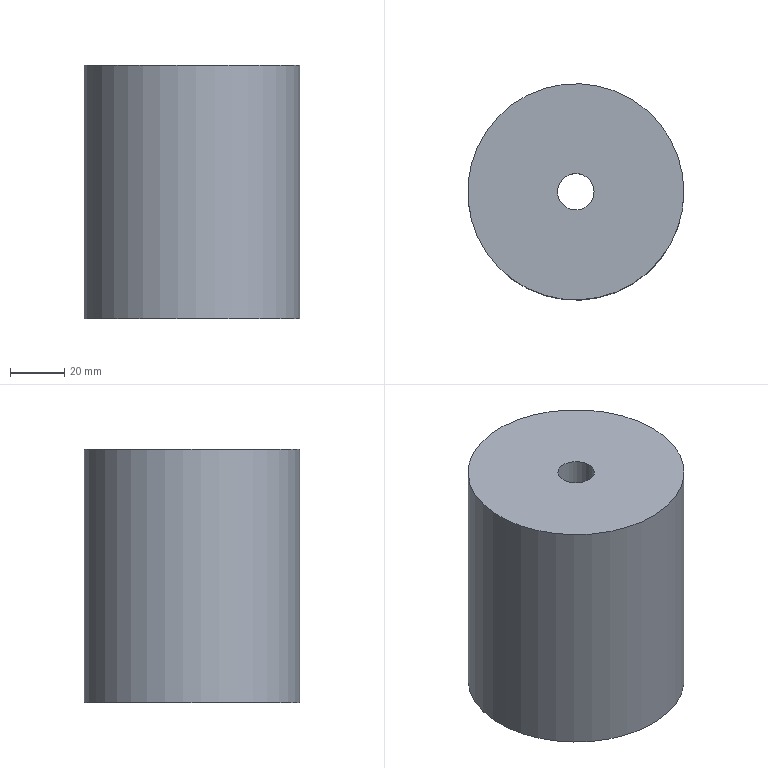Part | NX | features solid 2 | 1 solid | 6 faces | box 80 x 80 x 94 mm | volume 448095 mm3 | plane 3 | cylinder 3 | commonest cylinder face diameters 13.5 x1 20 x1 80 x1
STEP:
#1=CARTESIAN_POINT('',(295.,-607.5,101.));
#2=VERTEX_POINT('',#1);
#3=CARTESIAN_POINT('',(255.,-607.5,101.));
#4=DIRECTION('',(0.,0.,1.));
#5=DIRECTION('',(1.,0.,0.));
#6=AXIS2_PLACEMENT_3D('',#3,#4,#5);
#7=CIRCLE('',#6,40.);
#8=EDGE_CURVE('',#2,#2,#7,.T.);
#9=ORIENTED_EDGE('',*,*,#8,.T.);
#10=EDGE_LOOP('',(#9));
#11=FACE_BOUND('',#10,.T.);
#12=CARTESIAN_POINT('',(261.75,-607.5,101.));
#13=VERTEX_POINT('',#12);
#14=CARTESIAN_POINT('',(255.,-607.5,101.));
#15=DIRECTION('',(0.,0.,-1.));
#16=DIRECTION('',(1.,0.,0.));
#17=AXIS2_PLACEMENT_3D('',#14,#15,#16);
#18=CIRCLE('',#17,6.75);
#19=EDGE_CURVE('',#13,#13,#18,.T.);
#20=ORIENTED_EDGE('',*,*,#19,.T.);
#21=EDGE_LOOP('',(#20));
#22=FACE_BOUND('',#21,.T.);
#23=CARTESIAN_POINT('',(332.5,193.,101.));
#24=DIRECTION('',(0.,0.,1.));
#25=DIRECTION('',(-1.,0.,0.));
#26=AXIS2_PLACEMENT_3D('',#23,#24,#25);
#27=PLANE('',#26);
#28=ADVANCED_FACE('',(#11,#22),#27,.T.);
#29=ORIENTED_EDGE('',*,*,#8,.F.);
#30=EDGE_LOOP('',(#29));
#31=FACE_BOUND('',#30,.T.);
#32=CARTESIAN_POINT('',(295.,-607.5,7.));
#33=VERTEX_POINT('',#32);
#34=CARTESIAN_POINT('',(255.,-607.5,7.));
#35=DIRECTION('',(0.,0.,1.));
#36=DIRECTION('',(1.,0.,0.));
#37=AXIS2_PLACEMENT_3D('',#34,#35,#36);
#38=CIRCLE('',#37,40.);
#39=EDGE_CURVE('',#33,#33,#38,.T.);
#40=ORIENTED_EDGE('',*,*,#39,.T.);
#41=EDGE_LOOP('',(#40));
#42=FACE_BOUND('',#41,.T.);
#43=CARTESIAN_POINT('',(255.,-607.5,47.));
#44=DIRECTION('',(0.,0.,-1.));
#45=DIRECTION('',(1.,0.,0.));
#46=AXIS2_PLACEMENT_3D('',#43,#44,#45);
#47=CYLINDRICAL_SURFACE('',#46,40.);
#48=ADVANCED_FACE('',(#31,#42),#47,.T.);
#49=CARTESIAN_POINT('',(265.,-607.5,7.));
#50=VERTEX_POINT('',#49);
#51=CARTESIAN_POINT('',(255.,-607.5,7.));
#52=DIRECTION('',(0.,0.,1.));
#53=DIRECTION('',(1.,0.,0.));
#54=AXIS2_PLACEMENT_3D('',#51,#52,#53);
#55=CIRCLE('',#54,10.);
#56=EDGE_CURVE('',#50,#50,#55,.T.);
#57=ORIENTED_EDGE('',*,*,#56,.T.);
#58=EDGE_LOOP('',(#57));
#59=FACE_BOUND('',#58,.T.);
#60=ORIENTED_EDGE('',*,*,#39,.F.);
#61=EDGE_LOOP('',(#60));
#62=FACE_BOUND('',#61,.T.);
#63=CARTESIAN_POINT('',(255.,-607.5,7.));
#64=DIRECTION('',(0.,0.,1.));
#65=DIRECTION('',(-1.,0.,0.));
#66=AXIS2_PLACEMENT_3D('',#63,#64,#65);
#67=PLANE('',#66);
#68=ADVANCED_FACE('',(#59,#62),#67,.F.);
#69=CARTESIAN_POINT('',(261.75,-607.5,71.));
#70=VERTEX_POINT('',#69);
#71=CARTESIAN_POINT('',(255.,-607.5,71.));
#72=DIRECTION('',(0.,0.,1.));
#73=DIRECTION('',(1.,0.,0.));
#74=AXIS2_PLACEMENT_3D('',#71,#72,#73);
#75=CIRCLE('',#74,6.75);
#76=EDGE_CURVE('',#70,#70,#75,.T.);
#77=ORIENTED_EDGE('',*,*,#76,.F.);
#78=EDGE_LOOP('',(#77));
#79=FACE_BOUND('',#78,.T.);
#80=ORIENTED_EDGE('',*,*,#19,.F.);
#81=EDGE_LOOP('',(#80));
#82=FACE_BOUND('',#81,.T.);
#83=CARTESIAN_POINT('',(255.,-607.5,7.));
#84=DIRECTION('',(0.,0.,1.));
#85=DIRECTION('',(-1.,0.,0.));
#86=AXIS2_PLACEMENT_3D('',#83,#84,#85);
#87=CYLINDRICAL_SURFACE('',#86,6.75);
#88=ADVANCED_FACE('',(#79,#82),#87,.F.);
#89=ORIENTED_EDGE('',*,*,#76,.T.);
#90=EDGE_LOOP('',(#89));
#91=FACE_BOUND('',#90,.T.);
#92=CARTESIAN_POINT('',(265.,-607.5,71.));
#93=VERTEX_POINT('',#92);
#94=CARTESIAN_POINT('',(255.,-607.5,71.));
#95=DIRECTION('',(0.,0.,1.));
#96=DIRECTION('',(1.,0.,0.));
#97=AXIS2_PLACEMENT_3D('',#94,#95,#96);
#98=CIRCLE('',#97,10.);
#99=EDGE_CURVE('',#93,#93,#98,.T.);
#100=ORIENTED_EDGE('',*,*,#99,.F.);
#101=EDGE_LOOP('',(#100));
#102=FACE_BOUND('',#101,.T.);
#103=CARTESIAN_POINT('',(282.5,193.,71.));
#104=DIRECTION('',(0.,0.,1.));
#105=DIRECTION('',(-1.,0.,0.));
#106=AXIS2_PLACEMENT_3D('',#103,#104,#105);
#107=PLANE('',#106);
#108=ADVANCED_FACE('',(#91,#102),#107,.F.);
#109=ORIENTED_EDGE('',*,*,#99,.T.);
#110=EDGE_LOOP('',(#109));
#111=FACE_BOUND('',#110,.T.);
#112=ORIENTED_EDGE('',*,*,#56,.F.);
#113=EDGE_LOOP('',(#112));
#114=FACE_BOUND('',#113,.T.);
#115=CARTESIAN_POINT('',(255.,-607.5,7.));
#116=DIRECTION('',(0.,0.,1.));
#117=DIRECTION('',(-1.,0.,0.));
#118=AXIS2_PLACEMENT_3D('',#115,#116,#117);
#119=CYLINDRICAL_SURFACE('',#118,10.);
#120=ADVANCED_FACE('',(#111,#114),#119,.F.);
#121=CLOSED_SHELL('',(#28,#48,#68,#88,#108,#120));
#122=MANIFOLD_SOLID_BREP('',#121);
#123=(LENGTH_UNIT()NAMED_UNIT(*)SI_UNIT(.MILLI.,.METRE.));
#124=UNCERTAINTY_MEASURE_WITH_UNIT(LENGTH_MEASURE(0.00001),#123,'','');
#125=(NAMED_UNIT(*)PLANE_ANGLE_UNIT()SI_UNIT($,.RADIAN.));
#126=(NAMED_UNIT(*)SI_UNIT($,.STERADIAN.)SOLID_ANGLE_UNIT());
#127=(GEOMETRIC_REPRESENTATION_CONTEXT(3)GLOBAL_UNCERTAINTY_ASSIGNED_CONTEXT((#124))GLOBAL_UNIT_ASSIGNED_CONTEXT((#123,#125,#126))REPRESENTATION_CONTEXT('',''));
#128=ADVANCED_BREP_SHAPE_REPRESENTATION('',(#122),#127);